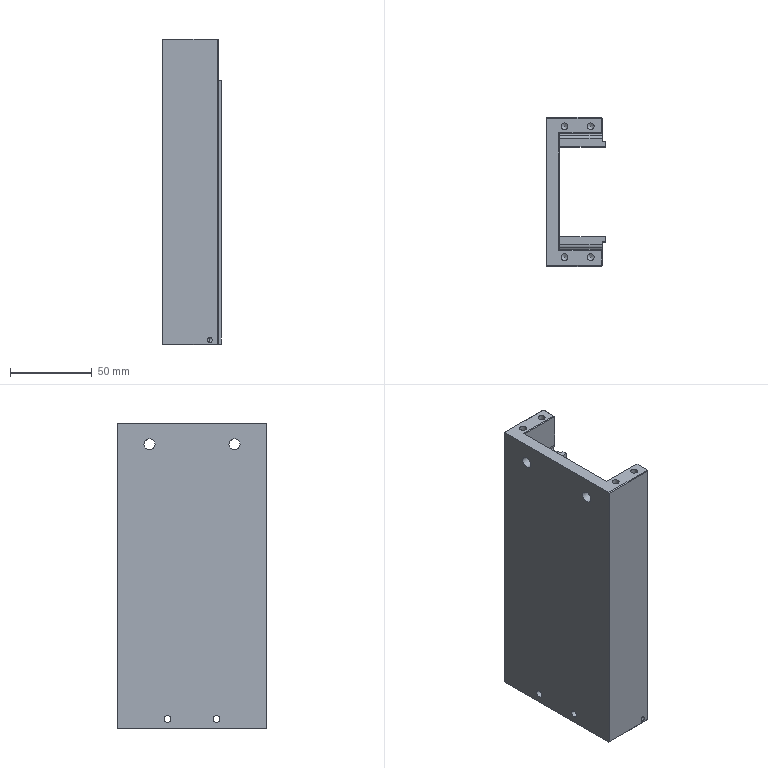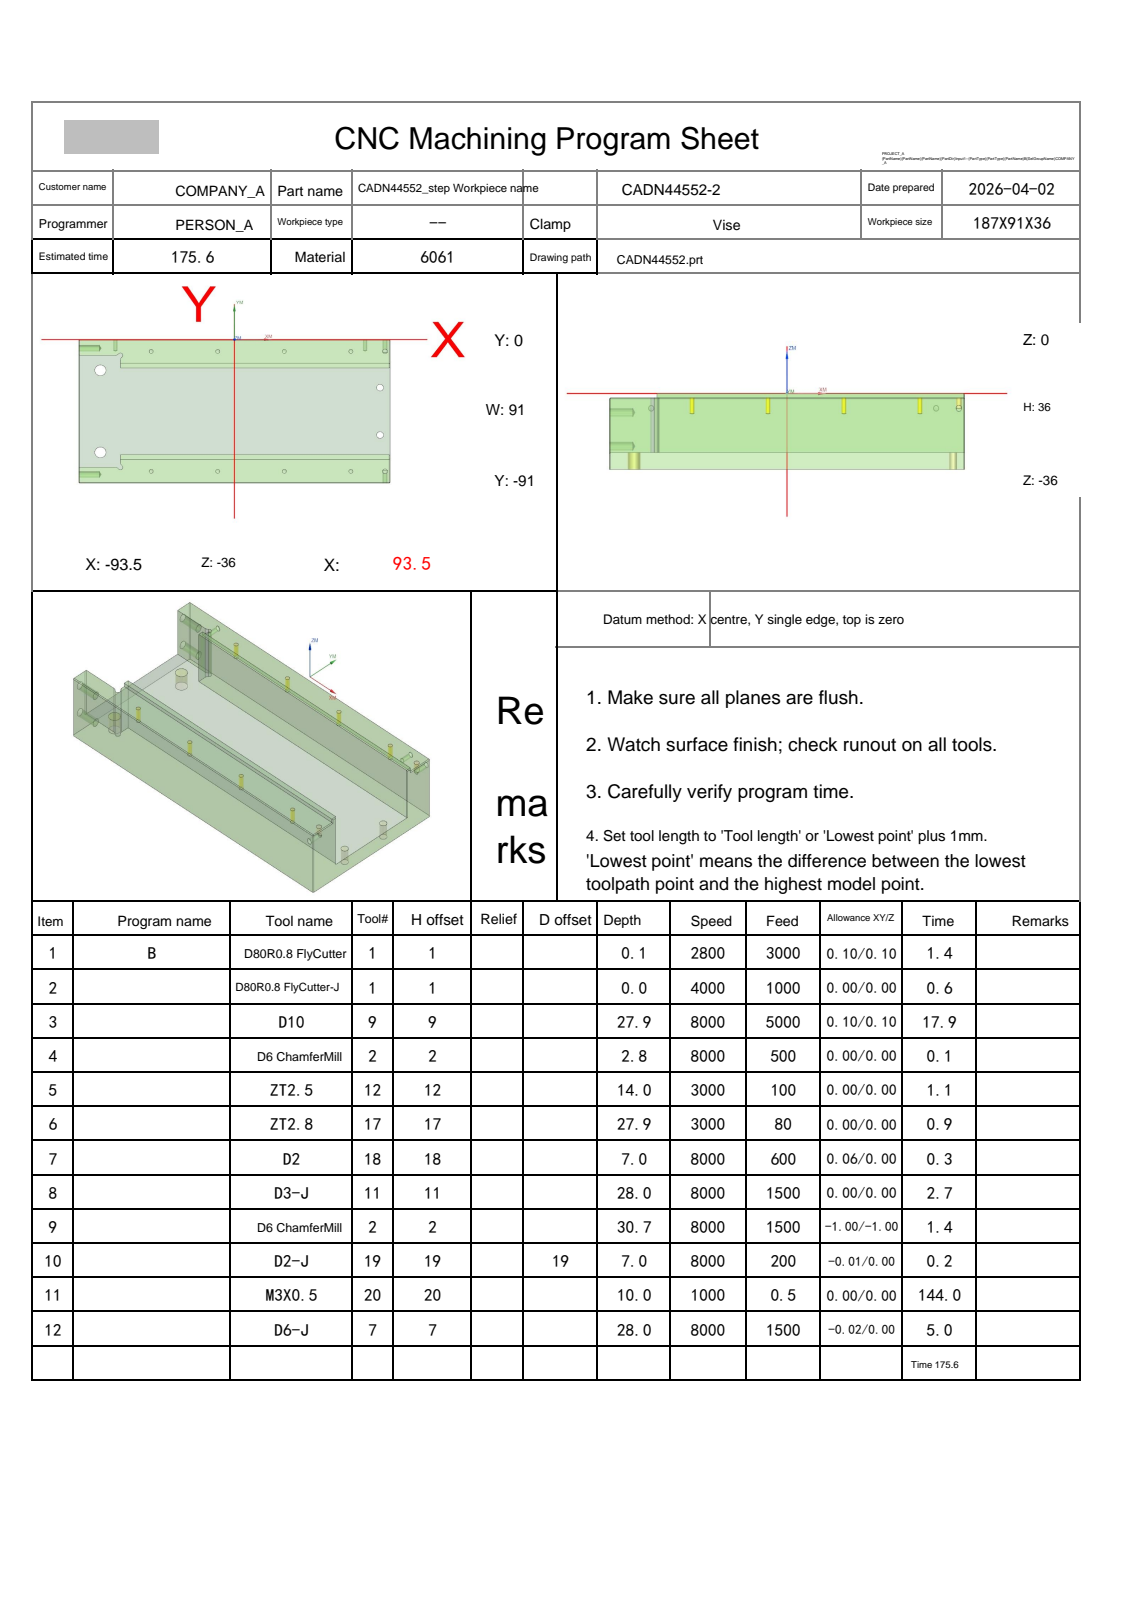NC program | NX | posted by the shop | part box 36 x 91 x 187 mm
Lines 128 to 1288 of 12140:
N3 T09 M06
(D10  D=10. R=0. H=09 ce=0.10 di=0.10)
G00 G90 G54 X-101. Y-45.5 M03 S8000
G43 H09 Z13.5
M08
Z.906
G01 Z-.594 F5000.
X-97.9
Y-12.312
X-95.112 Y-15.1
X-73.6
Y-23.1
X95.112
X98.4 Y-19.812
Y-71.188
X95.112 Y-67.9
X-73.6
Y-75.9
X-95.112
X-97.9 Y-78.688
Y-48.535
G02 X-97.455 Y-47.703 I1. J0.0
G01 X-90.845 Y-43.297
G03 X-90.4 Y-42.465 I-.555 J.832
G01 Y-23.597
G02 X-89.403 Y-22.6 I1. J-.003
G01 X-86.16
X-86.103 Y-22.591
X-86.069 Y-22.638
X-85.981 Y-22.726
X-85.93 Y-22.786
X-85.851
G02 X-83.6 Y-24.638 I-.166 J-2.495
G01 X-81.377 Y-33.006
G02 X-81.293 Y-33.648 I-2.416 J-.642
X-83.793 Y-36.148 I-2.5 J0.0
X-86.209 Y-34.29 I0.0 J2.5
G01 X-88.432 Y-25.922
G02 X-88.516 Y-25.28 I2.416 J.642
X-86.155 Y-22.784 I2.5 J0.0
G01 X-86.102 Y-22.791
X-86.071 Y-22.747
X-85.987 Y-22.661
X-85.927 Y-22.597
X-85.84 Y-22.6
X-82.082
G02 X-81.087 Y-23.538 I-.003 J-1.
G03 X-73.6 Y-30.6 I7.487 J.438
G01 X89.903
G02 X90.9 Y-31.597 I-.003 J-1.
G01 Y-59.403
G02 X89.903 Y-60.4 I-1. J.003
G01 X-73.6
G03 X-81.087 Y-67.462 I0.0 J-7.5
G02 X-82.082 Y-68.4 I-.998 J.062
G01 X-85.873
X-85.93 Y-68.409
X-85.964 Y-68.362
X-86.051 Y-68.274
X-86.103 Y-68.214
X-86.182
G02 X-88.516 Y-65.72 I.166 J2.495
X-88.432 Y-65.078 I2.5 J0.0
G01 X-86.209 Y-56.71
G02 X-83.793 Y-54.852 I2.416 J-.642
X-81.293 Y-57.352 I0.0 J-2.5
X-81.377 Y-57.994 I-2.5 J0.0
G01 X-83.6 Y-66.362
G02 X-85.877 Y-68.216 I-2.416 J.642
G01 X-85.931 Y-68.208
X-85.961 Y-68.253
X-86.046 Y-68.339
X-86.105 Y-68.403
X-86.192 Y-68.4
X-89.403
G02 X-90.4 Y-67.403 I.003 J1.
G01 Y-48.535
G02 X-89.955 Y-47.703 I1. J0.0
G01 X-83.345 Y-43.297
G03 X-82.9 Y-42.465 I-.555 J.832
G01 Y-36.775
G02 X-81.9 Y-35.779 I1. J-.004
X-81.384 Y-35.922 I0.0 J-1.
G03 X-73.6 Y-38.1 I7.784 J12.822
G01 X82.404
G02 X83.4 Y-39.096 I-.004 J-1.
G01 Y-51.904
G02 X82.404 Y-52.9 I-1. J.004
G01 X-73.6
G03 X-81.384 Y-55.078 I0.0 J-15.
G02 X-81.9 Y-55.221 I-.516 J.857
X-82.9 Y-54.225 I0.0 J1.
G01 Y-48.163
G02 X-82.608 Y-47.457 I1. J0.0
G01 X-78.635 Y-43.476
G03 X-78.371 Y-43.007 I-.708 J.706
G02 X-77.4 Y-42.245 I.971 J-.237
G01 X-77.219 Y-42.261
G03 X-73.6 Y-42.6 I3.619 J19.161
G01 X77.904
G02 X78.9 Y-43.596 I-.004 J-1.
G01 Y-47.404
G02 X77.904 Y-48.4 I-1. J.004
G01 X-73.6
G03 X-77.219 Y-48.739 I0.0 J-19.5
G01 X-77.4 Y-48.755
G02 X-78.4 Y-47.759 I0.0 J1.
G01 Y-45.5
Y-45.
X-81.4
Z.906
G00 X-101. Y-45.5
Z.313
G01 Z-1.187
X-97.9
Y-12.312
X-95.112 Y-15.1
X-73.6
Y-23.1
X95.112
X98.4 Y-19.812
Y-71.188
X95.112 Y-67.9
X-73.6
Y-75.9
X-95.112
X-97.9 Y-78.688
Y-48.535
G02 X-97.455 Y-47.703 I1. J0.0
G01 X-90.845 Y-43.297
G03 X-90.4 Y-42.465 I-.555 J.832
G01 Y-23.597
G02 X-89.403 Y-22.6 I1. J-.003
G01 X-86.16
X-86.103 Y-22.591
X-86.069 Y-22.638
X-85.981 Y-22.726
X-85.93 Y-22.786
X-85.851
G02 X-83.6 Y-24.638 I-.166 J-2.495
G01 X-81.377 Y-33.006
G02 X-81.293 Y-33.648 I-2.416 J-.642
X-83.793 Y-36.148 I-2.5 J0.0
X-86.209 Y-34.29 I0.0 J2.5
G01 X-88.432 Y-25.922
G02 X-88.516 Y-25.28 I2.416 J.642
X-86.155 Y-22.784 I2.5 J0.0
G01 X-86.102 Y-22.791
X-86.071 Y-22.747
X-85.987 Y-22.661
X-85.927 Y-22.597
X-85.84 Y-22.6
X-82.082
G02 X-81.087 Y-23.538 I-.003 J-1.
G03 X-73.6 Y-30.6 I7.487 J.438
G01 X89.903
G02 X90.9 Y-31.597 I-.003 J-1.
G01 Y-59.403
G02 X89.903 Y-60.4 I-1. J.003
G01 X-73.6
G03 X-81.087 Y-67.462 I0.0 J-7.5
G02 X-82.082 Y-68.4 I-.998 J.062
G01 X-85.873
X-85.93 Y-68.409
X-85.964 Y-68.362
X-86.051 Y-68.274
X-86.103 Y-68.214
X-86.182
G02 X-88.516 Y-65.72 I.166 J2.495
X-88.432 Y-65.078 I2.5 J0.0
G01 X-86.209 Y-56.71
G02 X-83.793 Y-54.852 I2.416 J-.642
X-81.293 Y-57.352 I0.0 J-2.5
X-81.377 Y-57.994 I-2.5 J0.0
G01 X-83.6 Y-66.362
G02 X-85.877 Y-68.216 I-2.416 J.642
G01 X-85.931 Y-68.208
X-85.961 Y-68.253
X-86.046 Y-68.339
X-86.105 Y-68.403
X-86.192 Y-68.4
X-89.403
G02 X-90.4 Y-67.403 I.003 J1.
G01 Y-48.535
G02 X-89.955 Y-47.703 I1. J0.0
G01 X-83.345 Y-43.297
G03 X-82.9 Y-42.465 I-.555 J.832
G01 Y-36.775
G02 X-81.9 Y-35.779 I1. J-.004
X-81.384 Y-35.922 I0.0 J-1.
G03 X-73.6 Y-38.1 I7.784 J12.822
G01 X82.404
G02 X83.4 Y-39.096 I-.004 J-1.
G01 Y-51.904
G02 X82.404 Y-52.9 I-1. J.004
G01 X-73.6
G03 X-81.384 Y-55.078 I0.0 J-15.
G02 X-81.9 Y-55.221 I-.516 J.857
X-82.9 Y-54.225 I0.0 J1.
G01 Y-48.163
G02 X-82.608 Y-47.457 I1. J0.0
G01 X-78.635 Y-43.476
G03 X-78.371 Y-43.007 I-.708 J.706
G02 X-77.4 Y-42.245 I.971 J-.237
G01 X-77.219 Y-42.261
G03 X-73.6 Y-42.6 I3.619 J19.161
G01 X77.904
G02 X78.9 Y-43.596 I-.004 J-1.
G01 Y-47.404
G02 X77.904 Y-48.4 I-1. J.004
G01 X-73.6
G03 X-77.219 Y-48.739 I0.0 J-19.5
G01 X-77.4 Y-48.755
G02 X-78.4 Y-47.759 I0.0 J1.
G01 Y-45.5
Y-45.
X-81.4
Z.313
G00 X-101. Y-45.5
Z-.281
G01 Z-1.781
X-97.9
Y-12.312
X-95.112 Y-15.1
X-73.6
Y-23.1
X95.112
X98.4 Y-19.812
Y-71.188
X95.112 Y-67.9
X-73.6
Y-75.9
X-95.112
X-97.9 Y-78.688
Y-48.535
G02 X-97.455 Y-47.703 I1. J0.0
G01 X-90.845 Y-43.297
G03 X-90.4 Y-42.465 I-.555 J.832
G01 Y-23.597
G02 X-89.403 Y-22.6 I1. J-.003
G01 X-86.16
X-86.103 Y-22.591
X-86.069 Y-22.638
X-85.981 Y-22.726
X-85.93 Y-22.786
X-85.851
G02 X-83.6 Y-24.638 I-.166 J-2.495
G01 X-81.377 Y-33.006
G02 X-81.293 Y-33.648 I-2.416 J-.642
X-83.793 Y-36.148 I-2.5 J0.0
X-86.209 Y-34.29 I0.0 J2.5
G01 X-88.432 Y-25.922
G02 X-88.516 Y-25.28 I2.416 J.642
X-86.155 Y-22.784 I2.5 J0.0
G01 X-86.102 Y-22.791
X-86.071 Y-22.747
X-85.987 Y-22.661
X-85.927 Y-22.597
X-85.84 Y-22.6
X-82.082
G02 X-81.087 Y-23.538 I-.003 J-1.
G03 X-73.6 Y-30.6 I7.487 J.438
G01 X89.903
G02 X90.9 Y-31.597 I-.003 J-1.
G01 Y-59.403
G02 X89.903 Y-60.4 I-1. J.003
G01 X-73.6
G03 X-81.087 Y-67.462 I0.0 J-7.5
G02 X-82.082 Y-68.4 I-.998 J.062
G01 X-85.873
X-85.93 Y-68.409
X-85.964 Y-68.362
X-86.051 Y-68.274
X-86.103 Y-68.214
X-86.182
G02 X-88.516 Y-65.72 I.166 J2.495
X-88.432 Y-65.078 I2.5 J0.0
G01 X-86.209 Y-56.71
G02 X-83.793 Y-54.852 I2.416 J-.642
X-81.293 Y-57.352 I0.0 J-2.5
X-81.377 Y-57.994 I-2.5 J0.0
G01 X-83.6 Y-66.362
G02 X-85.877 Y-68.216 I-2.416 J.642
G01 X-85.931 Y-68.208
X-85.961 Y-68.253
X-86.046 Y-68.339
X-86.105 Y-68.403
X-86.192 Y-68.4
X-89.403
G02 X-90.4 Y-67.403 I.003 J1.
G01 Y-48.535
G02 X-89.955 Y-47.703 I1. J0.0
G01 X-83.345 Y-43.297
G03 X-82.9 Y-42.465 I-.555 J.832
G01 Y-36.775
G02 X-81.9 Y-35.779 I1. J-.004
X-81.384 Y-35.922 I0.0 J-1.
G03 X-73.6 Y-38.1 I7.784 J12.822
G01 X82.404
G02 X83.4 Y-39.096 I-.004 J-1.
G01 Y-51.904
G02 X82.404 Y-52.9 I-1. J.004
G01 X-73.6
G03 X-81.384 Y-55.078 I0.0 J-15.
G02 X-81.9 Y-55.221 I-.516 J.857
X-82.9 Y-54.225 I0.0 J1.
G01 Y-48.163
G02 X-82.608 Y-47.457 I1. J0.0
G01 X-78.635 Y-43.476
G03 X-78.371 Y-43.007 I-.708 J.706
G02 X-77.4 Y-42.245 I.971 J-.237
G01 X-77.219 Y-42.261
G03 X-73.6 Y-42.6 I3.619 J19.161
G01 X77.904
G02 X78.9 Y-43.596 I-.004 J-1.
G01 Y-47.404
G02 X77.904 Y-48.4 I-1. J.004
G01 X-73.6
G03 X-77.219 Y-48.739 I0.0 J-19.5
G01 X-77.4 Y-48.755
G02 X-78.4 Y-47.759 I0.0 J1.
G01 Y-45.5
Y-45.
X-81.4
Z-.281
G00 X-101. Y-45.5
Z-.874
G01 Z-2.374
X-97.9
Y-12.312
X-95.112 Y-15.1
X-73.6
Y-23.1
X95.112
X98.4 Y-19.812
Y-71.188
X95.112 Y-67.9
X-73.6
Y-75.9
X-95.112
X-97.9 Y-78.688
Y-48.535
G02 X-97.455 Y-47.703 I1. J0.0
G01 X-90.845 Y-43.297
G03 X-90.4 Y-42.465 I-.555 J.832
G01 Y-23.597
G02 X-89.403 Y-22.6 I1. J-.003
G01 X-86.16
X-86.103 Y-22.591
X-86.069 Y-22.638
X-85.981 Y-22.726
X-85.93 Y-22.786
X-85.851
G02 X-83.6 Y-24.638 I-.166 J-2.495
G01 X-81.377 Y-33.006
G02 X-81.293 Y-33.648 I-2.416 J-.642
X-83.793 Y-36.148 I-2.5 J0.0
X-86.209 Y-34.29 I0.0 J2.5
G01 X-88.432 Y-25.922
G02 X-88.516 Y-25.28 I2.416 J.642
X-86.155 Y-22.784 I2.5 J0.0
G01 X-86.102 Y-22.791
X-86.071 Y-22.747
X-85.987 Y-22.661
X-85.927 Y-22.597
X-85.84 Y-22.6
X-82.082
G02 X-81.087 Y-23.538 I-.003 J-1.
G03 X-73.6 Y-30.6 I7.487 J.438
G01 X89.903
G02 X90.9 Y-31.597 I-.003 J-1.
G01 Y-59.403
G02 X89.903 Y-60.4 I-1. J.003
G01 X-73.6
G03 X-81.087 Y-67.462 I0.0 J-7.5
G02 X-82.082 Y-68.4 I-.998 J.062
G01 X-85.873
X-85.93 Y-68.409
X-85.964 Y-68.362
X-86.051 Y-68.274
X-86.103 Y-68.214
X-86.182
G02 X-88.516 Y-65.72 I.166 J2.495
X-88.432 Y-65.078 I2.5 J0.0
G01 X-86.209 Y-56.71
G02 X-83.793 Y-54.852 I2.416 J-.642
X-81.293 Y-57.352 I0.0 J-2.5
X-81.377 Y-57.994 I-2.5 J0.0
G01 X-83.6 Y-66.362
G02 X-85.877 Y-68.216 I-2.416 J.642
G01 X-85.931 Y-68.208
X-85.961 Y-68.253
X-86.046 Y-68.339
X-86.105 Y-68.403
X-86.192 Y-68.4
X-89.403
G02 X-90.4 Y-67.403 I.003 J1.
G01 Y-48.535
G02 X-89.955 Y-47.703 I1. J0.0
G01 X-83.345 Y-43.297
G03 X-82.9 Y-42.465 I-.555 J.832
G01 Y-36.775
G02 X-81.9 Y-35.779 I1. J-.004
X-81.384 Y-35.922 I0.0 J-1.
G03 X-73.6 Y-38.1 I7.784 J12.822
G01 X82.404
G02 X83.4 Y-39.096 I-.004 J-1.
G01 Y-51.904
G02 X82.404 Y-52.9 I-1. J.004
G01 X-73.6
G03 X-81.384 Y-55.078 I0.0 J-15.
G02 X-81.9 Y-55.221 I-.516 J.857
X-82.9 Y-54.225 I0.0 J1.
G01 Y-48.163
G02 X-82.608 Y-47.457 I1. J0.0
G01 X-78.635 Y-43.476
G03 X-78.371 Y-43.007 I-.708 J.706
G02 X-77.4 Y-42.245 I.971 J-.237
G01 X-77.219 Y-42.261
G03 X-73.6 Y-42.6 I3.619 J19.161
G01 X77.904
G02 X78.9 Y-43.596 I-.004 J-1.
G01 Y-47.404
G02 X77.904 Y-48.4 I-1. J.004
G01 X-73.6
G03 X-77.219 Y-48.739 I0.0 J-19.5
G01 X-77.4 Y-48.755
G02 X-78.4 Y-47.759 I0.0 J1.
G01 Y-45.5
Y-45.
X-81.4
Z-.874
G00 X-101. Y-45.5
Z-1.468
G01 Z-2.968
X-97.9
Y-12.312
X-95.112 Y-15.1
X-73.6
Y-23.1
X95.112
X98.4 Y-19.812
Y-71.188
X95.112 Y-67.9
X-73.6
Y-75.9
X-95.112
X-97.9 Y-78.688
Y-48.535
G02 X-97.455 Y-47.703 I1. J0.0
G01 X-90.845 Y-43.297
G03 X-90.4 Y-42.465 I-.555 J.832
G01 Y-23.597
G02 X-89.403 Y-22.6 I1. J-.003
G01 X-86.16
X-86.103 Y-22.591
X-86.069 Y-22.638
X-85.981 Y-22.726
X-85.93 Y-22.786
X-85.851
G02 X-83.6 Y-24.638 I-.166 J-2.495
G01 X-81.377 Y-33.006
G02 X-81.293 Y-33.648 I-2.416 J-.642
X-83.793 Y-36.148 I-2.5 J0.0
X-86.209 Y-34.29 I0.0 J2.5
G01 X-88.432 Y-25.922
G02 X-88.516 Y-25.28 I2.416 J.642
X-86.155 Y-22.784 I2.5 J0.0
G01 X-86.102 Y-22.791
X-86.071 Y-22.747
X-85.987 Y-22.661
X-85.927 Y-22.597
X-85.84 Y-22.6
X-82.082
G02 X-81.087 Y-23.538 I-.003 J-1.
G03 X-73.6 Y-30.6 I7.487 J.438
G01 X89.903
G02 X90.9 Y-31.597 I-.003 J-1.
G01 Y-59.403
G02 X89.903 Y-60.4 I-1. J.003
G01 X-73.6
G03 X-81.087 Y-67.462 I0.0 J-7.5
G02 X-82.082 Y-68.4 I-.998 J.062
G01 X-85.873
X-85.93 Y-68.409
X-85.964 Y-68.362
X-86.051 Y-68.274
X-86.103 Y-68.214
X-86.182
G02 X-88.516 Y-65.72 I.166 J2.495
X-88.432 Y-65.078 I2.5 J0.0
G01 X-86.209 Y-56.71
G02 X-83.793 Y-54.852 I2.416 J-.642
X-81.293 Y-57.352 I0.0 J-2.5
X-81.377 Y-57.994 I-2.5 J0.0
G01 X-83.6 Y-66.362
G02 X-85.877 Y-68.216 I-2.416 J.642
G01 X-85.931 Y-68.208
X-85.961 Y-68.253
X-86.046 Y-68.339
X-86.105 Y-68.403
X-86.192 Y-68.4
X-89.403
G02 X-90.4 Y-67.403 I.003 J1.
G01 Y-48.535
G02 X-89.955 Y-47.703 I1. J0.0
G01 X-83.345 Y-43.297
G03 X-82.9 Y-42.465 I-.555 J.832
G01 Y-36.775
G02 X-81.9 Y-35.779 I1. J-.004
X-81.384 Y-35.922 I0.0 J-1.
G03 X-73.6 Y-38.1 I7.784 J12.822
G01 X82.404
G02 X83.4 Y-39.096 I-.004 J-1.
G01 Y-51.904
G02 X82.404 Y-52.9 I-1. J.004
G01 X-73.6
G03 X-81.384 Y-55.078 I0.0 J-15.
G02 X-81.9 Y-55.221 I-.516 J.857
X-82.9 Y-54.225 I0.0 J1.
G01 Y-48.163
G02 X-82.608 Y-47.457 I1. J0.0
G01 X-78.635 Y-43.476
G03 X-78.371 Y-43.007 I-.708 J.706
G02 X-77.4 Y-42.245 I.971 J-.237
G01 X-77.219 Y-42.261
G03 X-73.6 Y-42.6 I3.619 J19.161
G01 X77.904
G02 X78.9 Y-43.596 I-.004 J-1.
G01 Y-47.404
G02 X77.904 Y-48.4 I-1. J.004
G01 X-73.6
G03 X-77.219 Y-48.739 I0.0 J-19.5
G01 X-77.4 Y-48.755
G02 X-78.4 Y-47.759 I0.0 J1.
G01 Y-45.5
Y-45.
X-81.4
Z-1.468
G00 X-101. Y-45.5
Z-2.062
G01 Z-3.562
X-97.9
Y-12.312
X-95.112 Y-15.1
X-73.6
Y-23.1
X95.112
X98.4 Y-19.812
Y-71.188
X95.112 Y-67.9
X-73.6
Y-75.9
X-95.112
X-97.9 Y-78.688
Y-48.535
G02 X-97.455 Y-47.703 I1. J0.0
G01 X-90.845 Y-43.297
G03 X-90.4 Y-42.465 I-.555 J.832
G01 Y-23.597
G02 X-89.403 Y-22.6 I1. J-.003
G01 X-86.16
X-86.103 Y-22.591
X-86.069 Y-22.638
X-85.981 Y-22.726
X-85.93 Y-22.786
X-85.851
G02 X-83.6 Y-24.638 I-.166 J-2.495
G01 X-81.377 Y-33.006
G02 X-81.293 Y-33.648 I-2.416 J-.642
X-83.793 Y-36.148 I-2.5 J0.0
X-86.209 Y-34.29 I0.0 J2.5
G01 X-88.432 Y-25.922
G02 X-88.516 Y-25.28 I2.416 J.642
X-86.155 Y-22.784 I2.5 J0.0
G01 X-86.102 Y-22.791
X-86.071 Y-22.747
X-85.987 Y-22.661
X-85.927 Y-22.597
X-85.84 Y-22.6
X-82.082
G02 X-81.087 Y-23.538 I-.003 J-1.
G03 X-73.6 Y-30.6 I7.487 J.438
G01 X89.903
G02 X90.9 Y-31.597 I-.003 J-1.
G01 Y-59.403
G02 X89.903 Y-60.4 I-1. J.003
G01 X-73.6
G03 X-81.087 Y-67.462 I0.0 J-7.5
G02 X-82.082 Y-68.4 I-.998 J.062
G01 X-85.873
X-85.93 Y-68.409
X-85.964 Y-68.362
X-86.051 Y-68.274
X-86.103 Y-68.214
X-86.182
G02 X-88.516 Y-65.72 I.166 J2.495
X-88.432 Y-65.078 I2.5 J0.0
G01 X-86.209 Y-56.71
G02 X-83.793 Y-54.852 I2.416 J-.642
X-81.293 Y-57.352 I0.0 J-2.5
X-81.377 Y-57.994 I-2.5 J0.0
G01 X-83.6 Y-66.362
G02 X-85.877 Y-68.216 I-2.416 J.642
G01 X-85.931 Y-68.208
X-85.961 Y-68.253
X-86.046 Y-68.339
X-86.105 Y-68.403
X-86.192 Y-68.4
X-89.403
G02 X-90.4 Y-67.403 I.003 J1.
G01 Y-48.535
G02 X-89.955 Y-47.703 I1. J0.0
G01 X-83.345 Y-43.297
G03 X-82.9 Y-42.465 I-.555 J.832
G01 Y-36.775
G02 X-81.9 Y-35.779 I1. J-.004
X-81.384 Y-35.922 I0.0 J-1.
G03 X-73.6 Y-38.1 I7.784 J12.822
G01 X82.404
G02 X83.4 Y-39.096 I-.004 J-1.
G01 Y-51.904
G02 X82.404 Y-52.9 I-1. J.004
G01 X-73.6
G03 X-81.384 Y-55.078 I0.0 J-15.
G02 X-81.9 Y-55.221 I-.516 J.857
X-82.9 Y-54.225 I0.0 J1.
G01 Y-48.163
G02 X-82.608 Y-47.457 I1. J0.0
G01 X-78.635 Y-43.476
G03 X-78.371 Y-43.007 I-.708 J.706
G02 X-77.4 Y-42.245 I.971 J-.237
G01 X-77.219 Y-42.261
G03 X-73.6 Y-42.6 I3.619 J19.161
G01 X77.904
G02 X78.9 Y-43.596 I-.004 J-1.
G01 Y-47.404
G02 X77.904 Y-48.4 I-1. J.004
G01 X-73.6
G03 X-77.219 Y-48.739 I0.0 J-19.5
G01 X-77.4 Y-48.755
G02 X-78.4 Y-47.759 I0.0 J1.
G01 Y-45.5
Y-45.
X-81.4
Z-2.062
G00 X-101. Y-45.5
Z-2.655
G01 Z-4.155
X-97.9
Y-12.312
X-95.112 Y-15.1
X-73.6
Y-23.1
X95.112
X98.4 Y-19.812
Y-71.188
X95.112 Y-67.9
X-73.6
Y-75.9
X-95.112
X-97.9 Y-78.688
Y-48.535
G02 X-97.455 Y-47.703 I1. J0.0
G01 X-90.845 Y-43.297
G03 X-90.4 Y-42.465 I-.555 J.832
G01 Y-23.597
G02 X-89.403 Y-22.6 I1. J-.003
G01 X-86.16
X-86.103 Y-22.591
X-86.069 Y-22.638
X-85.981 Y-22.726
X-85.93 Y-22.786
X-85.851
G02 X-83.6 Y-24.638 I-.166 J-2.495
G01 X-81.377 Y-33.006
G02 X-81.293 Y-33.648 I-2.416 J-.642
X-83.793 Y-36.148 I-2.5 J0.0
X-86.209 Y-34.29 I0.0 J2.5
G01 X-88.432 Y-25.922
G02 X-88.516 Y-25.28 I2.416 J.642
X-86.155 Y-22.784 I2.5 J0.0
G01 X-86.102 Y-22.791
X-86.071 Y-22.747
X-85.987 Y-22.661
X-85.927 Y-22.597
X-85.84 Y-22.6
X-82.082
G02 X-81.087 Y-23.538 I-.003 J-1.
G03 X-73.6 Y-30.6 I7.487 J.438
G01 X89.903
G02 X90.9 Y-31.597 I-.003 J-1.
G01 Y-59.403
G02 X89.903 Y-60.4 I-1. J.003
G01 X-73.6
G03 X-81.087 Y-67.462 I0.0 J-7.5
G02 X-82.082 Y-68.4 I-.998 J.062
G01 X-85.873
X-85.93 Y-68.409
X-85.964 Y-68.362
X-86.051 Y-68.274
X-86.103 Y-68.214
X-86.182
G02 X-88.516 Y-65.72 I.166 J2.495
X-88.432 Y-65.078 I2.5 J0.0
G01 X-86.209 Y-56.71
G02 X-83.793 Y-54.852 I2.416 J-.642
X-81.293 Y-57.352 I0.0 J-2.5
X-81.377 Y-57.994 I-2.5 J0.0
G01 X-83.6 Y-66.362
G02 X-85.877 Y-68.216 I-2.416 J.642
G01 X-85.931 Y-68.208
X-85.961 Y-68.253
X-86.046 Y-68.339
X-86.105 Y-68.403
X-86.192 Y-68.4
X-89.403
G02 X-90.4 Y-67.403 I.003 J1.
G01 Y-48.535
G02 X-89.955 Y-47.703 I1. J0.0
G01 X-83.345 Y-43.297
G03 X-82.9 Y-42.465 I-.555 J.832
G01 Y-36.775
G02 X-81.9 Y-35.779 I1. J-.004
X-81.384 Y-35.922 I0.0 J-1.
G03 X-73.6 Y-38.1 I7.784 J12.822
G01 X82.404
G02 X83.4 Y-39.096 I-.004 J-1.
G01 Y-51.904
G02 X82.404 Y-52.9 I-1. J.004
G01 X-73.6
G03 X-81.384 Y-55.078 I0.0 J-15.
G02 X-81.9 Y-55.221 I-.516 J.857
X-82.9 Y-54.225 I0.0 J1.
G01 Y-48.163
G02 X-82.608 Y-47.457 I1. J0.0
G01 X-78.635 Y-43.476
G03 X-78.371 Y-43.007 I-.708 J.706
G02 X-77.4 Y-42.245 I.971 J-.237
G01 X-77.219 Y-42.261
G03 X-73.6 Y-42.6 I3.619 J19.161
G01 X77.904
G02 X78.9 Y-43.596 I-.004 J-1.
G01 Y-47.404
G02 X77.904 Y-48.4 I-1. J.004
G01 X-73.6
G03 X-77.219 Y-48.739 I0.0 J-19.5
G01 X-77.4 Y-48.755
G02 X-78.4 Y-47.759 I0.0 J1.
G01 Y-45.5
Y-45.
X-81.4
Z-2.655
G00 X-101. Y-45.5
Z-3.249
G01 Z-4.749
X-97.9
Y-12.312
X-95.112 Y-15.1
X-73.6
Y-23.1
X95.112
X98.4 Y-19.812
Y-71.188
X95.112 Y-67.9
X-73.6
Y-75.9
X-95.112
X-97.9 Y-78.688
Y-48.535
G02 X-97.455 Y-47.703 I1. J0.0
G01 X-90.845 Y-43.297
G03 X-90.4 Y-42.465 I-.555 J.832
G01 Y-23.597
G02 X-89.403 Y-22.6 I1. J-.003
G01 X-86.16
X-86.103 Y-22.591
X-86.069 Y-22.638
X-85.981 Y-22.726
X-85.93 Y-22.786
X-85.851
G02 X-83.6 Y-24.638 I-.166 J-2.495
G01 X-81.377 Y-33.006
G02 X-81.293 Y-33.648 I-2.416 J-.642
X-83.793 Y-36.148 I-2.5 J0.0
X-86.209 Y-34.29 I0.0 J2.5
G01 X-88.432 Y-25.922
G02 X-88.516 Y-25.28 I2.416 J.642
X-86.155 Y-22.784 I2.5 J0.0
G01 X-86.102 Y-22.791
X-86.071 Y-22.747
X-85.987 Y-22.661
X-85.927 Y-22.597
X-85.84 Y-22.6
X-82.082
G02 X-81.087 Y-23.538 I-.003 J-1.
G03 X-73.6 Y-30.6 I7.487 J.438
G01 X89.903
G02 X90.9 Y-31.597 I-.003 J-1.
G01 Y-59.403
G02 X89.903 Y-60.4 I-1. J.003
G01 X-73.6
G03 X-81.087 Y-67.462 I0.0 J-7.5
G02 X-82.082 Y-68.4 I-.998 J.062
G01 X-85.873
X-85.93 Y-68.409
X-85.964 Y-68.362
X-86.051 Y-68.274
X-86.103 Y-68.214
X-86.182
G02 X-88.516 Y-65.72 I.166 J2.495
X-88.432 Y-65.078 I2.5 J0.0
G01 X-86.209 Y-56.71
G02 X-83.793 Y-54.852 I2.416 J-.642
X-81.293 Y-57.352 I0.0 J-2.5
X-81.377 Y-57.994 I-2.5 J0.0
G01 X-83.6 Y-66.362
G02 X-85.877 Y-68.216 I-2.416 J.642
G01 X-85.931 Y-68.208
X-85.961 Y-68.253
X-86.046 Y-68.339
X-86.105 Y-68.403
X-86.192 Y-68.4
X-89.403
G02 X-90.4 Y-67.403 I.003 J1.
G01 Y-48.535
G02 X-89.955 Y-47.703 I1. J0.0
G01 X-83.345 Y-43.297
G03 X-82.9 Y-42.465 I-.555 J.832
G01 Y-36.775
G02 X-81.9 Y-35.779 I1. J-.004
X-81.384 Y-35.922 I0.0 J-1.
G03 X-73.6 Y-38.1 I7.784 J12.822
G01 X82.404
G02 X83.4 Y-39.096 I-.004 J-1.
G01 Y-51.904
G02 X82.404 Y-52.9 I-1. J.004
G01 X-73.6
G03 X-81.384 Y-55.078 I0.0 J-15.
G02 X-81.9 Y-55.221 I-.516 J.857
X-82.9 Y-54.225 I0.0 J1.
G01 Y-48.163
G02 X-82.608 Y-47.457 I1. J0.0
G01 X-78.635 Y-43.476
G03 X-78.371 Y-43.007 I-.708 J.706
G02 X-77.4 Y-42.245 I.971 J-.237
G01 X-77.219 Y-42.261
G03 X-73.6 Y-42.6 I3.619 J19.161
G01 X77.904
G02 X78.9 Y-43.596 I-.004 J-1.
G01 Y-47.404
G02 X77.904 Y-48.4 I-1. J.004
G01 X-73.6
G03 X-77.219 Y-48.739 I0.0 J-19.5
G01 X-77.4 Y-48.755
G02 X-78.4 Y-47.759 I0.0 J1.
G01 Y-45.5
Y-45.
X-81.4
Z-3.249
G00 X-101. Y-45.5
Z-3.843
G01 Z-5.343
X-97.9
Y-12.312
X-95.112 Y-15.1
X-73.6
Y-23.1
X95.112
X98.4 Y-19.812
Y-71.188
X95.112 Y-67.9
X-73.6
Y-75.9
X-95.112
X-97.9 Y-78.688
Y-48.535
G02 X-97.455 Y-47.703 I1. J0.0
G01 X-90.845 Y-43.297
G03 X-90.4 Y-42.465 I-.555 J.832
G01 Y-23.597
G02 X-89.403 Y-22.6 I1. J-.003
G01 X-86.16
X-86.103 Y-22.591
X-86.069 Y-22.638
X-85.981 Y-22.726
X-85.93 Y-22.786
X-85.851
G02 X-83.6 Y-24.638 I-.166 J-2.495
G01 X-81.377 Y-33.006
G02 X-81.293 Y-33.648 I-2.416 J-.642
X-83.793 Y-36.148 I-2.5 J0.0
X-86.209 Y-34.29 I0.0 J2.5
G01 X-88.432 Y-25.922
G02 X-88.516 Y-25.28 I2.416 J.642
X-86.155 Y-22.784 I2.5 J0.0
G01 X-86.102 Y-22.791
X-86.071 Y-22.747
X-85.987 Y-22.661
X-85.927 Y-22.597
X-85.84 Y-22.6
X-82.082
G02 X-81.087 Y-23.538 I-.003 J-1.
G03 X-73.6 Y-30.6 I7.487 J.438
G01 X89.903
G02 X90.9 Y-31.597 I-.003 J-1.
G01 Y-59.403
G02 X89.903 Y-60.4 I-1. J.003
G01 X-73.6
G03 X-81.087 Y-67.462 I0.0 J-7.5
G02 X-82.082 Y-68.4 I-.998 J.062
G01 X-85.873
X-85.93 Y-68.409
X-85.964 Y-68.362
X-86.051 Y-68.274
X-86.103 Y-68.214
X-86.182
G02 X-88.516 Y-65.72 I.166 J2.495
X-88.432 Y-65.078 I2.5 J0.0
G01 X-86.209 Y-56.71
G02 X-83.793 Y-54.852 I2.416 J-.642
X-81.293 Y-57.352 I0.0 J-2.5
X-81.377 Y-57.994 I-2.5 J0.0
G01 X-83.6 Y-66.362
G02 X-85.877 Y-68.216 I-2.416 J.642
G01 X-85.931 Y-68.208
X-85.961 Y-68.253
X-86.046 Y-68.339
X-86.105 Y-68.403
X-86.192 Y-68.4
X-89.403
G02 X-90.4 Y-67.403 I.003 J1.
G01 Y-48.535
G02 X-89.955 Y-47.703 I1. J0.0
G01 X-83.345 Y-43.297
G03 X-82.9 Y-42.465 I-.555 J.832
G01 Y-36.775
G02 X-81.9 Y-35.779 I1. J-.004
X-81.384 Y-35.922 I0.0 J-1.
G03 X-73.6 Y-38.1 I7.784 J12.822
G01 X82.404
G02 X83.4 Y-39.096 I-.004 J-1.
G01 Y-51.904
G02 X82.404 Y-52.9 I-1. J.004
G01 X-73.6
G03 X-81.384 Y-55.078 I0.0 J-15.
G02 X-81.9 Y-55.221 I-.516 J.857
X-82.9 Y-54.225 I0.0 J1.
G01 Y-48.163
G02 X-82.608 Y-47.457 I1. J0.0
G01 X-78.635 Y-43.476
G03 X-78.371 Y-43.007 I-.708 J.706
G02 X-77.4 Y-42.245 I.971 J-.237
G01 X-77.219 Y-42.261
G03 X-73.6 Y-42.6 I3.619 J19.161
G01 X77.904
G02 X78.9 Y-43.596 I-.004 J-1.
G01 Y-47.404
G02 X77.904 Y-48.4 I-1. J.004
G01 X-73.6
G03 X-77.219 Y-48.739 I0.0 J-19.5
G01 X-77.4 Y-48.755
G02 X-78.4 Y-47.759 I0.0 J1.
G01 Y-45.5
Y-45.
X-81.4
Z-3.843
G00 X-101. Y-45.5
Z-4.436
G01 Z-5.936
X-97.9
Y-12.312
X-95.112 Y-15.1
X-73.6
Y-23.1
X95.112
X98.4 Y-19.812
Y-71.188
X95.112 Y-67.9
X-73.6
Y-75.9
X-95.112
X-97.9 Y-78.688
Y-48.535
G02 X-97.455 Y-47.703 I1. J0.0
G01 X-90.845 Y-43.297
G03 X-90.4 Y-42.465 I-.555 J.832
G01 Y-23.597
G02 X-89.403 Y-22.6 I1. J-.003
G01 X-86.16
X-86.103 Y-22.591
X-86.069 Y-22.638
X-85.981 Y-22.726
X-85.93 Y-22.786
X-85.851
G02 X-83.6 Y-24.638 I-.166 J-2.495
G01 X-81.377 Y-33.006
G02 X-81.293 Y-33.648 I-2.416 J-.642
X-83.793 Y-36.148 I-2.5 J0.0
X-86.209 Y-34.29 I0.0 J2.5
G01 X-88.432 Y-25.922
G02 X-88.516 Y-25.28 I2.416 J.642
X-86.155 Y-22.784 I2.5 J0.0
G01 X-86.102 Y-22.791
X-86.071 Y-22.747
X-85.987 Y-22.661
X-85.927 Y-22.597
X-85.84 Y-22.6
X-82.082
G02 X-81.087 Y-23.538 I-.003 J-1.
G03 X-73.6 Y-30.6 I7.487 J.438
G01 X89.903
G02 X90.9 Y-31.597 I-.003 J-1.
G01 Y-59.403
G02 X89.903 Y-60.4 I-1. J.003
G01 X-73.6
G03 X-81.087 Y-67.462 I0.0 J-7.5
G02 X-82.082 Y-68.4 I-.998 J.062
G01 X-85.873
X-85.93 Y-68.409
X-85.964 Y-68.362
X-86.051 Y-68.274
X-86.103 Y-68.214
X-86.182
G02 X-88.516 Y-65.72 I.166 J2.495
X-88.432 Y-65.078 I2.5 J0.0
G01 X-86.209 Y-56.71
G02 X-83.793 Y-54.852 I2.416 J-.642
X-81.293 Y-57.352 I0.0 J-2.5
X-81.377 Y-57.994 I-2.5 J0.0
G01 X-83.6 Y-66.362
G02 X-85.877 Y-68.216 I-2.416 J.642
G01 X-85.931 Y-68.208
X-85.961 Y-68.253
X-86.046 Y-68.339
X-86.105 Y-68.403
X-86.192 Y-68.4
X-89.403
G02 X-90.4 Y-67.403 I.003 J1.
G01 Y-48.535
G02 X-89.955 Y-47.703 I1. J0.0
G01 X-83.345 Y-43.297
G03 X-82.9 Y-42.465 I-.555 J.832
G01 Y-36.775
G02 X-81.9 Y-35.779 I1. J-.004
X-81.384 Y-35.922 I0.0 J-1.
G03 X-73.6 Y-38.1 I7.784 J12.822
G01 X82.404
G02 X83.4 Y-39.096 I-.004 J-1.
G01 Y-51.904
G02 X82.404 Y-52.9 I-1. J.004
G01 X-73.6
G03 X-81.384 Y-55.078 I0.0 J-15.
G02 X-81.9 Y-55.221 I-.516 J.857
X-82.9 Y-54.225 I0.0 J1.
G01 Y-48.163
G02 X-82.608 Y-47.457 I1. J0.0
G01 X-78.635 Y-43.476
G03 X-78.371 Y-43.007 I-.708 J.706
G02 X-77.4 Y-42.245 I.971 J-.237
G01 X-77.219 Y-42.261
G03 X-73.6 Y-42.6 I3.619 J19.161
G01 X77.904
G02 X78.9 Y-43.596 I-.004 J-1.
G01 Y-47.404
G02 X77.904 Y-48.4 I-1. J.004
G01 X-73.6
G03 X-77.219 Y-48.739 I0.0 J-19.5
G01 X-77.4 Y-48.755
G02 X-78.4 Y-47.759 I0.0 J1.
G01 Y-45.5
Y-45.
X-81.4
Z-4.436
G00 X-101. Y-45.5
Z-5.03
G01 Z-6.53
X-97.9
Y-12.312
X-95.112 Y-15.1
X-73.6
Y-23.1
X95.112
X98.4 Y-19.812
Y-71.188
X95.112 Y-67.9
X-73.6
Y-75.9
X-95.112
X-97.9 Y-78.688
Y-48.535
G02 X-97.455 Y-47.703 I1. J0.0
G01 X-90.845 Y-43.297
G03 X-90.4 Y-42.465 I-.555 J.832
G01 Y-23.597
G02 X-89.403 Y-22.6 I1. J-.003
G01 X-86.16
X-86.103 Y-22.591
X-86.069 Y-22.638
X-85.981 Y-22.726
X-85.93 Y-22.786
X-85.851
G02 X-83.6 Y-24.638 I-.166 J-2.495
G01 X-81.377 Y-33.006
G02 X-81.293 Y-33.648 I-2.416 J-.642
X-83.793 Y-36.148 I-2.5 J0.0
X-86.209 Y-34.29 I0.0 J2.5
G01 X-88.432 Y-25.922
G02 X-88.516 Y-25.28 I2.416 J.642
X-86.155 Y-22.784 I2.5 J0.0
G01 X-86.102 Y-22.791
X-86.071 Y-22.747
X-85.987 Y-22.661
X-85.927 Y-22.597
X-85.84 Y-22.6
X-82.082
G02 X-81.087 Y-23.538 I-.003 J-1.
G03 X-73.6 Y-30.6 I7.487 J.438
G01 X89.903
G02 X90.9 Y-31.597 I-.003 J-1.
G01 Y-59.403
G02 X89.903 Y-60.4 I-1. J.003
G01 X-73.6
G03 X-81.087 Y-67.462 I0.0 J-7.5
G02 X-82.082 Y-68.4 I-.998 J.062
G01 X-85.873
X-85.93 Y-68.409
X-85.964 Y-68.362
X-86.051 Y-68.274
X-86.103 Y-68.214
X-86.182
G02 X-88.516 Y-65.72 I.166 J2.495
X-88.432 Y-65.078 I2.5 J0.0
G01 X-86.209 Y-56.71
G02 X-83.793 Y-54.852 I2.416 J-.642
X-81.293 Y-57.352 I0.0 J-2.5
X-81.377 Y-57.994 I-2.5 J0.0
G01 X-83.6 Y-66.362
G02 X-85.877 Y-68.216 I-2.416 J.642
G01 X-85.931 Y-68.208
X-85.961 Y-68.253
X-86.046 Y-68.339
X-86.105 Y-68.403
X-86.192 Y-68.4
X-89.403
G02 X-90.4 Y-67.403 I.003 J1.
G01 Y-48.535
G02 X-89.955 Y-47.703 I1. J0.0
G01 X-83.345 Y-43.297
G03 X-82.9 Y-42.465 I-.555 J.832
G01 Y-36.775
G02 X-81.9 Y-35.779 I1. J-.004
X-81.384 Y-35.922 I0.0 J-1.
G03 X-73.6 Y-38.1 I7.784 J12.822
G01 X82.404
G02 X83.4 Y-39.096 I-.004 J-1.
G01 Y-51.904
G02 X82.404 Y-52.9 I-1. J.004
G01 X-73.6
G03 X-81.384 Y-55.078 I0.0 J-15.
G02 X-81.9 Y-55.221 I-.516 J.857